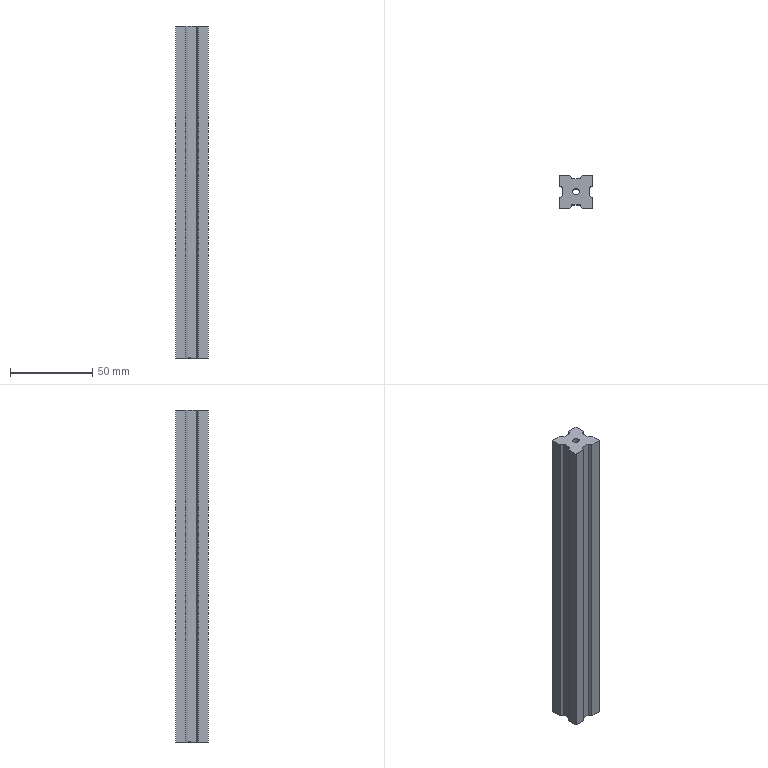Part | SolidWorks | features CirPattern 1, Extrusion 1, ICE 1 | 1 solid | 24 faces | box 20 x 20 x 202 mm | volume 68046 mm3 | plane 22 | cylinder 2 | commonest cylinder face diameters 3.889 x2
STEP:
#1=CARTESIAN_POINT('',(-1.944,0.,101.));
#2=VERTEX_POINT('',#1);
#3=CARTESIAN_POINT('',(1.944,0.,101.));
#4=VERTEX_POINT('',#3);
#5=CARTESIAN_POINT('',(0.,0.,101.));
#6=DIRECTION('',(0.,0.,1.));
#7=DIRECTION('',(1.,0.,0.));
#8=AXIS2_PLACEMENT_3D('',#5,#6,#7);
#9=CIRCLE('',#8,1.944);
#10=EDGE_CURVE('',#2,#4,#9,.T.);
#11=ORIENTED_EDGE('',*,*,#10,.T.);
#12=CARTESIAN_POINT('',(1.944,0.,-101.));
#13=VERTEX_POINT('',#12);
#14=CARTESIAN_POINT('',(1.944,0.,101.));
#15=DIRECTION('',(0.,0.,-1.));
#16=VECTOR('',#15,1000.);
#17=LINE('',#14,#16);
#18=EDGE_CURVE('',#4,#13,#17,.T.);
#19=ORIENTED_EDGE('',*,*,#18,.T.);
#20=CARTESIAN_POINT('',(-1.944,0.,-101.));
#21=VERTEX_POINT('',#20);
#22=CARTESIAN_POINT('',(0.,0.,-101.));
#23=DIRECTION('',(0.,0.,1.));
#24=DIRECTION('',(1.,0.,0.));
#25=AXIS2_PLACEMENT_3D('',#22,#23,#24);
#26=CIRCLE('',#25,1.944);
#27=EDGE_CURVE('',#21,#13,#26,.T.);
#28=ORIENTED_EDGE('',*,*,#27,.F.);
#29=CARTESIAN_POINT('',(-1.944,0.,101.));
#30=DIRECTION('',(0.,0.,-1.));
#31=VECTOR('',#30,1000.);
#32=LINE('',#29,#31);
#33=EDGE_CURVE('',#2,#21,#32,.T.);
#34=ORIENTED_EDGE('',*,*,#33,.F.);
#35=EDGE_LOOP('',(#11,#19,#28,#34));
#36=FACE_OUTER_BOUND('',#35,.T.);
#37=CARTESIAN_POINT('',(0.,0.,101.));
#38=DIRECTION('',(0.,0.,-1.));
#39=DIRECTION('',(-1.,0.,0.));
#40=AXIS2_PLACEMENT_3D('',#37,#38,#39);
#41=CYLINDRICAL_SURFACE('',#40,1.944);
#42=ADVANCED_FACE('',(#36),#41,.F.);
#43=CARTESIAN_POINT('',(-10.,3.694,101.));
#44=VERTEX_POINT('',#43);
#45=CARTESIAN_POINT('',(-10.,3.694,-101.));
#46=VERTEX_POINT('',#45);
#47=CARTESIAN_POINT('',(-10.,3.694,355.963));
#48=DIRECTION('',(0.,0.,-1.));
#49=VECTOR('',#48,1000.);
#50=LINE('',#47,#49);
#51=EDGE_CURVE('',#44,#46,#50,.T.);
#52=ORIENTED_EDGE('',*,*,#51,.F.);
#53=CARTESIAN_POINT('',(-10.,10.,101.));
#54=VERTEX_POINT('',#53);
#55=CARTESIAN_POINT('',(-10.,-10.,101.));
#56=DIRECTION('',(0.,-1.,0.));
#57=VECTOR('',#56,1000.);
#58=LINE('',#55,#57);
#59=EDGE_CURVE('',#54,#44,#58,.T.);
#60=ORIENTED_EDGE('',*,*,#59,.F.);
#61=CARTESIAN_POINT('',(-10.,10.,-101.));
#62=VERTEX_POINT('',#61);
#63=CARTESIAN_POINT('',(-10.,10.,101.));
#64=DIRECTION('',(0.,0.,-1.));
#65=VECTOR('',#64,1000.);
#66=LINE('',#63,#65);
#67=EDGE_CURVE('',#54,#62,#66,.T.);
#68=ORIENTED_EDGE('',*,*,#67,.T.);
#69=CARTESIAN_POINT('',(-10.,-10.,-101.));
#70=DIRECTION('',(0.,-1.,0.));
#71=VECTOR('',#70,1000.);
#72=LINE('',#69,#71);
#73=EDGE_CURVE('',#62,#46,#72,.T.);
#74=ORIENTED_EDGE('',*,*,#73,.T.);
#75=EDGE_LOOP('',(#52,#60,#68,#74));
#76=FACE_OUTER_BOUND('',#75,.T.);
#77=CARTESIAN_POINT('',(-10.,-10.,101.));
#78=DIRECTION('',(1.,0.,0.));
#79=DIRECTION('',(0.,0.,-1.));
#80=AXIS2_PLACEMENT_3D('',#77,#78,#79);
#81=PLANE('',#80);
#82=ADVANCED_FACE('',(#76),#81,.F.);
#83=ORIENTED_EDGE('',*,*,#10,.F.);
#84=CARTESIAN_POINT('',(0.,0.,101.));
#85=DIRECTION('',(0.,0.,1.));
#86=DIRECTION('',(1.,0.,0.));
#87=AXIS2_PLACEMENT_3D('',#84,#85,#86);
#88=CIRCLE('',#87,1.944);
#89=EDGE_CURVE('',#4,#2,#88,.T.);
#90=ORIENTED_EDGE('',*,*,#89,.F.);
#91=EDGE_LOOP('',(#83,#90));
#92=FACE_BOUND('',#91,.T.);
#93=CARTESIAN_POINT('',(-7.931,2.5,101.));
#94=VERTEX_POINT('',#93);
#95=CARTESIAN_POINT('',(-7.931,-2.5,101.));
#96=VERTEX_POINT('',#95);
#97=CARTESIAN_POINT('',(-7.931,0.,101.));
#98=DIRECTION('',(0.,-1.,0.));
#99=VECTOR('',#98,1000.);
#100=LINE('',#97,#99);
#101=EDGE_CURVE('',#94,#96,#100,.T.);
#102=ORIENTED_EDGE('',*,*,#101,.T.);
#103=CARTESIAN_POINT('',(-10.,-3.694,101.));
#104=VERTEX_POINT('',#103);
#105=CARTESIAN_POINT('',(-0.9003,1.559,101.));
#106=DIRECTION('',(-0.866,-0.5,0.));
#107=VECTOR('',#106,1000.);
#108=LINE('',#105,#107);
#109=EDGE_CURVE('',#96,#104,#108,.T.);
#110=ORIENTED_EDGE('',*,*,#109,.T.);
#111=CARTESIAN_POINT('',(-10.,-10.,101.));
#112=VERTEX_POINT('',#111);
#113=CARTESIAN_POINT('',(-10.,-10.,101.));
#114=DIRECTION('',(0.,-1.,0.));
#115=VECTOR('',#114,1000.);
#116=LINE('',#113,#115);
#117=EDGE_CURVE('',#104,#112,#116,.T.);
#118=ORIENTED_EDGE('',*,*,#117,.T.);
#119=CARTESIAN_POINT('',(-3.694,-10.,101.));
#120=VERTEX_POINT('',#119);
#121=CARTESIAN_POINT('',(10.,-10.,101.));
#122=DIRECTION('',(1.,0.,0.));
#123=VECTOR('',#122,1000.);
#124=LINE('',#121,#123);
#125=EDGE_CURVE('',#112,#120,#124,.T.);
#126=ORIENTED_EDGE('',*,*,#125,.T.);
#127=CARTESIAN_POINT('',(-2.5,-7.931,101.));
#128=VERTEX_POINT('',#127);
#129=CARTESIAN_POINT('',(1.559,-0.9003,101.));
#130=DIRECTION('',(0.5,0.866,0.));
#131=VECTOR('',#130,1000.);
#132=LINE('',#129,#131);
#133=EDGE_CURVE('',#120,#128,#132,.T.);
#134=ORIENTED_EDGE('',*,*,#133,.T.);
#135=CARTESIAN_POINT('',(2.5,-7.931,101.));
#136=VERTEX_POINT('',#135);
#137=CARTESIAN_POINT('',(0.,-7.931,101.));
#138=DIRECTION('',(1.,0.,0.));
#139=VECTOR('',#138,1000.);
#140=LINE('',#137,#139);
#141=EDGE_CURVE('',#128,#136,#140,.T.);
#142=ORIENTED_EDGE('',*,*,#141,.T.);
#143=CARTESIAN_POINT('',(3.694,-10.,101.));
#144=VERTEX_POINT('',#143);
#145=CARTESIAN_POINT('',(-1.559,-0.9003,101.));
#146=DIRECTION('',(0.5,-0.866,0.));
#147=VECTOR('',#146,1000.);
#148=LINE('',#145,#147);
#149=EDGE_CURVE('',#136,#144,#148,.T.);
#150=ORIENTED_EDGE('',*,*,#149,.T.);
#151=CARTESIAN_POINT('',(10.,-10.,101.));
#152=VERTEX_POINT('',#151);
#153=CARTESIAN_POINT('',(10.,-10.,101.));
#154=DIRECTION('',(1.,0.,0.));
#155=VECTOR('',#154,1000.);
#156=LINE('',#153,#155);
#157=EDGE_CURVE('',#144,#152,#156,.T.);
#158=ORIENTED_EDGE('',*,*,#157,.T.);
#159=CARTESIAN_POINT('',(10.,-3.694,101.));
#160=VERTEX_POINT('',#159);
#161=CARTESIAN_POINT('',(10.,-10.,101.));
#162=DIRECTION('',(0.,1.,0.));
#163=VECTOR('',#162,1000.);
#164=LINE('',#161,#163);
#165=EDGE_CURVE('',#152,#160,#164,.T.);
#166=ORIENTED_EDGE('',*,*,#165,.T.);
#167=CARTESIAN_POINT('',(7.931,-2.5,101.));
#168=VERTEX_POINT('',#167);
#169=CARTESIAN_POINT('',(0.9003,1.559,101.));
#170=DIRECTION('',(-0.866,0.5,0.));
#171=VECTOR('',#170,1000.);
#172=LINE('',#169,#171);
#173=EDGE_CURVE('',#160,#168,#172,.T.);
#174=ORIENTED_EDGE('',*,*,#173,.T.);
#175=CARTESIAN_POINT('',(7.931,2.5,101.));
#176=VERTEX_POINT('',#175);
#177=CARTESIAN_POINT('',(7.931,0.,101.));
#178=DIRECTION('',(0.,1.,0.));
#179=VECTOR('',#178,1000.);
#180=LINE('',#177,#179);
#181=EDGE_CURVE('',#168,#176,#180,.T.);
#182=ORIENTED_EDGE('',*,*,#181,.T.);
#183=CARTESIAN_POINT('',(10.,3.694,101.));
#184=VERTEX_POINT('',#183);
#185=CARTESIAN_POINT('',(0.9003,-1.559,101.));
#186=DIRECTION('',(0.866,0.5,0.));
#187=VECTOR('',#186,1000.);
#188=LINE('',#185,#187);
#189=EDGE_CURVE('',#176,#184,#188,.T.);
#190=ORIENTED_EDGE('',*,*,#189,.T.);
#191=CARTESIAN_POINT('',(10.,10.,101.));
#192=VERTEX_POINT('',#191);
#193=CARTESIAN_POINT('',(10.,-10.,101.));
#194=DIRECTION('',(0.,1.,0.));
#195=VECTOR('',#194,1000.);
#196=LINE('',#193,#195);
#197=EDGE_CURVE('',#184,#192,#196,.T.);
#198=ORIENTED_EDGE('',*,*,#197,.T.);
#199=CARTESIAN_POINT('',(3.694,10.,101.));
#200=VERTEX_POINT('',#199);
#201=CARTESIAN_POINT('',(10.,10.,101.));
#202=DIRECTION('',(-1.,0.,0.));
#203=VECTOR('',#202,1000.);
#204=LINE('',#201,#203);
#205=EDGE_CURVE('',#192,#200,#204,.T.);
#206=ORIENTED_EDGE('',*,*,#205,.T.);
#207=CARTESIAN_POINT('',(2.5,7.931,101.));
#208=VERTEX_POINT('',#207);
#209=CARTESIAN_POINT('',(-1.559,0.9003,101.));
#210=DIRECTION('',(-0.5,-0.866,0.));
#211=VECTOR('',#210,1000.);
#212=LINE('',#209,#211);
#213=EDGE_CURVE('',#200,#208,#212,.T.);
#214=ORIENTED_EDGE('',*,*,#213,.T.);
#215=CARTESIAN_POINT('',(-2.5,7.931,101.));
#216=VERTEX_POINT('',#215);
#217=CARTESIAN_POINT('',(0.,7.931,101.));
#218=DIRECTION('',(-1.,0.,0.));
#219=VECTOR('',#218,1000.);
#220=LINE('',#217,#219);
#221=EDGE_CURVE('',#208,#216,#220,.T.);
#222=ORIENTED_EDGE('',*,*,#221,.T.);
#223=CARTESIAN_POINT('',(-3.694,10.,101.));
#224=VERTEX_POINT('',#223);
#225=CARTESIAN_POINT('',(1.559,0.9003,101.));
#226=DIRECTION('',(-0.5,0.866,0.));
#227=VECTOR('',#226,1000.);
#228=LINE('',#225,#227);
#229=EDGE_CURVE('',#216,#224,#228,.T.);
#230=ORIENTED_EDGE('',*,*,#229,.T.);
#231=CARTESIAN_POINT('',(10.,10.,101.));
#232=DIRECTION('',(-1.,0.,0.));
#233=VECTOR('',#232,1000.);
#234=LINE('',#231,#233);
#235=EDGE_CURVE('',#224,#54,#234,.T.);
#236=ORIENTED_EDGE('',*,*,#235,.T.);
#237=ORIENTED_EDGE('',*,*,#59,.T.);
#238=CARTESIAN_POINT('',(-0.9003,-1.559,101.));
#239=DIRECTION('',(0.866,-0.5,0.));
#240=VECTOR('',#239,1000.);
#241=LINE('',#238,#240);
#242=EDGE_CURVE('',#44,#94,#241,.T.);
#243=ORIENTED_EDGE('',*,*,#242,.T.);
#244=EDGE_LOOP('',(#102,#110,#118,#126,#134,#142,#150,#158,#166,#174,#182,#190,#198,#206,#214,#222,#230,#236,#237,#243));
#245=FACE_OUTER_BOUND('',#244,.T.);
#246=CARTESIAN_POINT('',(0.,0.,101.));
#247=DIRECTION('',(0.,0.,1.));
#248=DIRECTION('',(1.,0.,0.));
#249=AXIS2_PLACEMENT_3D('',#246,#247,#248);
#250=PLANE('',#249);
#251=ADVANCED_FACE('',(#92,#245),#250,.T.);
#252=ORIENTED_EDGE('',*,*,#27,.T.);
#253=CARTESIAN_POINT('',(0.,0.,-101.));
#254=DIRECTION('',(0.,0.,1.));
#255=DIRECTION('',(1.,0.,0.));
#256=AXIS2_PLACEMENT_3D('',#253,#254,#255);
#257=CIRCLE('',#256,1.944);
#258=EDGE_CURVE('',#13,#21,#257,.T.);
#259=ORIENTED_EDGE('',*,*,#258,.T.);
#260=EDGE_LOOP('',(#252,#259));
#261=FACE_BOUND('',#260,.T.);
#262=CARTESIAN_POINT('',(-7.931,-2.5,-101.));
#263=VERTEX_POINT('',#262);
#264=CARTESIAN_POINT('',(-10.,-3.694,-101.));
#265=VERTEX_POINT('',#264);
#266=CARTESIAN_POINT('',(-0.9003,1.559,-101.));
#267=DIRECTION('',(-0.866,-0.5,0.));
#268=VECTOR('',#267,1000.);
#269=LINE('',#266,#268);
#270=EDGE_CURVE('',#263,#265,#269,.T.);
#271=ORIENTED_EDGE('',*,*,#270,.F.);
#272=CARTESIAN_POINT('',(-7.931,2.5,-101.));
#273=VERTEX_POINT('',#272);
#274=CARTESIAN_POINT('',(-7.931,0.,-101.));
#275=DIRECTION('',(0.,-1.,0.));
#276=VECTOR('',#275,1000.);
#277=LINE('',#274,#276);
#278=EDGE_CURVE('',#273,#263,#277,.T.);
#279=ORIENTED_EDGE('',*,*,#278,.F.);
#280=CARTESIAN_POINT('',(-0.9003,-1.559,-101.));
#281=DIRECTION('',(0.866,-0.5,0.));
#282=VECTOR('',#281,1000.);
#283=LINE('',#280,#282);
#284=EDGE_CURVE('',#46,#273,#283,.T.);
#285=ORIENTED_EDGE('',*,*,#284,.F.);
#286=ORIENTED_EDGE('',*,*,#73,.F.);
#287=CARTESIAN_POINT('',(-3.694,10.,-101.));
#288=VERTEX_POINT('',#287);
#289=CARTESIAN_POINT('',(10.,10.,-101.));
#290=DIRECTION('',(-1.,0.,0.));
#291=VECTOR('',#290,1000.);
#292=LINE('',#289,#291);
#293=EDGE_CURVE('',#288,#62,#292,.T.);
#294=ORIENTED_EDGE('',*,*,#293,.F.);
#295=CARTESIAN_POINT('',(-2.5,7.931,-101.));
#296=VERTEX_POINT('',#295);
#297=CARTESIAN_POINT('',(1.559,0.9003,-101.));
#298=DIRECTION('',(-0.5,0.866,0.));
#299=VECTOR('',#298,1000.);
#300=LINE('',#297,#299);
#301=EDGE_CURVE('',#296,#288,#300,.T.);
#302=ORIENTED_EDGE('',*,*,#301,.F.);
#303=CARTESIAN_POINT('',(2.5,7.931,-101.));
#304=VERTEX_POINT('',#303);
#305=CARTESIAN_POINT('',(0.,7.931,-101.));
#306=DIRECTION('',(-1.,0.,0.));
#307=VECTOR('',#306,1000.);
#308=LINE('',#305,#307);
#309=EDGE_CURVE('',#304,#296,#308,.T.);
#310=ORIENTED_EDGE('',*,*,#309,.F.);
#311=CARTESIAN_POINT('',(3.694,10.,-101.));
#312=VERTEX_POINT('',#311);
#313=CARTESIAN_POINT('',(-1.559,0.9003,-101.));
#314=DIRECTION('',(-0.5,-0.866,0.));
#315=VECTOR('',#314,1000.);
#316=LINE('',#313,#315);
#317=EDGE_CURVE('',#312,#304,#316,.T.);
#318=ORIENTED_EDGE('',*,*,#317,.F.);
#319=CARTESIAN_POINT('',(10.,10.,-101.));
#320=VERTEX_POINT('',#319);
#321=CARTESIAN_POINT('',(10.,10.,-101.));
#322=DIRECTION('',(-1.,0.,0.));
#323=VECTOR('',#322,1000.);
#324=LINE('',#321,#323);
#325=EDGE_CURVE('',#320,#312,#324,.T.);
#326=ORIENTED_EDGE('',*,*,#325,.F.);
#327=CARTESIAN_POINT('',(10.,3.694,-101.));
#328=VERTEX_POINT('',#327);
#329=CARTESIAN_POINT('',(10.,-10.,-101.));
#330=DIRECTION('',(0.,1.,0.));
#331=VECTOR('',#330,1000.);
#332=LINE('',#329,#331);
#333=EDGE_CURVE('',#328,#320,#332,.T.);
#334=ORIENTED_EDGE('',*,*,#333,.F.);
#335=CARTESIAN_POINT('',(7.931,2.5,-101.));
#336=VERTEX_POINT('',#335);
#337=CARTESIAN_POINT('',(0.9003,-1.559,-101.));
#338=DIRECTION('',(0.866,0.5,0.));
#339=VECTOR('',#338,1000.);
#340=LINE('',#337,#339);
#341=EDGE_CURVE('',#336,#328,#340,.T.);
#342=ORIENTED_EDGE('',*,*,#341,.F.);
#343=CARTESIAN_POINT('',(7.931,-2.5,-101.));
#344=VERTEX_POINT('',#343);
#345=CARTESIAN_POINT('',(7.931,0.,-101.));
#346=DIRECTION('',(0.,1.,0.));
#347=VECTOR('',#346,1000.);
#348=LINE('',#345,#347);
#349=EDGE_CURVE('',#344,#336,#348,.T.);
#350=ORIENTED_EDGE('',*,*,#349,.F.);
#351=CARTESIAN_POINT('',(10.,-3.694,-101.));
#352=VERTEX_POINT('',#351);
#353=CARTESIAN_POINT('',(0.9003,1.559,-101.));
#354=DIRECTION('',(-0.866,0.5,0.));
#355=VECTOR('',#354,1000.);
#356=LINE('',#353,#355);
#357=EDGE_CURVE('',#352,#344,#356,.T.);
#358=ORIENTED_EDGE('',*,*,#357,.F.);
#359=CARTESIAN_POINT('',(10.,-10.,-101.));
#360=VERTEX_POINT('',#359);
#361=CARTESIAN_POINT('',(10.,-10.,-101.));
#362=DIRECTION('',(0.,1.,0.));
#363=VECTOR('',#362,1000.);
#364=LINE('',#361,#363);
#365=EDGE_CURVE('',#360,#352,#364,.T.);
#366=ORIENTED_EDGE('',*,*,#365,.F.);
#367=CARTESIAN_POINT('',(3.694,-10.,-101.));
#368=VERTEX_POINT('',#367);
#369=CARTESIAN_POINT('',(10.,-10.,-101.));
#370=DIRECTION('',(1.,0.,0.));
#371=VECTOR('',#370,1000.);
#372=LINE('',#369,#371);
#373=EDGE_CURVE('',#368,#360,#372,.T.);
#374=ORIENTED_EDGE('',*,*,#373,.F.);
#375=CARTESIAN_POINT('',(2.5,-7.931,-101.));
#376=VERTEX_POINT('',#375);
#377=CARTESIAN_POINT('',(-1.559,-0.9003,-101.));
#378=DIRECTION('',(0.5,-0.866,0.));
#379=VECTOR('',#378,1000.);
#380=LINE('',#377,#379);
#381=EDGE_CURVE('',#376,#368,#380,.T.);
#382=ORIENTED_EDGE('',*,*,#381,.F.);
#383=CARTESIAN_POINT('',(-2.5,-7.931,-101.));
#384=VERTEX_POINT('',#383);
#385=CARTESIAN_POINT('',(0.,-7.931,-101.));
#386=DIRECTION('',(1.,0.,0.));
#387=VECTOR('',#386,1000.);
#388=LINE('',#385,#387);
#389=EDGE_CURVE('',#384,#376,#388,.T.);
#390=ORIENTED_EDGE('',*,*,#389,.F.);
#391=CARTESIAN_POINT('',(-3.694,-10.,-101.));
#392=VERTEX_POINT('',#391);
#393=CARTESIAN_POINT('',(1.559,-0.9003,-101.));
#394=DIRECTION('',(0.5,0.866,0.));
#395=VECTOR('',#394,1000.);
#396=LINE('',#393,#395);
#397=EDGE_CURVE('',#392,#384,#396,.T.);
#398=ORIENTED_EDGE('',*,*,#397,.F.);
#399=CARTESIAN_POINT('',(-10.,-10.,-101.));
#400=VERTEX_POINT('',#399);
#401=CARTESIAN_POINT('',(10.,-10.,-101.));
#402=DIRECTION('',(1.,0.,0.));
#403=VECTOR('',#402,1000.);
#404=LINE('',#401,#403);
#405=EDGE_CURVE('',#400,#392,#404,.T.);
#406=ORIENTED_EDGE('',*,*,#405,.F.);
#407=CARTESIAN_POINT('',(-10.,-10.,-101.));
#408=DIRECTION('',(0.,-1.,0.));
#409=VECTOR('',#408,1000.);
#410=LINE('',#407,#409);
#411=EDGE_CURVE('',#265,#400,#410,.T.);
#412=ORIENTED_EDGE('',*,*,#411,.F.);
#413=EDGE_LOOP('',(#271,#279,#285,#286,#294,#302,#310,#318,#326,#334,#342,#350,#358,#366,#374,#382,#390,#398,#406,#412));
#414=FACE_OUTER_BOUND('',#413,.T.);
#415=CARTESIAN_POINT('',(0.,0.,-101.));
#416=DIRECTION('',(0.,0.,1.));
#417=DIRECTION('',(1.,0.,0.));
#418=AXIS2_PLACEMENT_3D('',#415,#416,#417);
#419=PLANE('',#418);
#420=ADVANCED_FACE('',(#261,#414),#419,.F.);
#421=CARTESIAN_POINT('',(-3.694,-10.,355.963));
#422=DIRECTION('',(0.,0.,-1.));
#423=VECTOR('',#422,1000.);
#424=LINE('',#421,#423);
#425=EDGE_CURVE('',#120,#392,#424,.T.);
#426=ORIENTED_EDGE('',*,*,#425,.F.);
#427=ORIENTED_EDGE('',*,*,#125,.F.);
#428=CARTESIAN_POINT('',(-10.,-10.,101.));
#429=DIRECTION('',(0.,0.,-1.));
#430=VECTOR('',#429,1000.);
#431=LINE('',#428,#430);
#432=EDGE_CURVE('',#112,#400,#431,.T.);
#433=ORIENTED_EDGE('',*,*,#432,.T.);
#434=ORIENTED_EDGE('',*,*,#405,.T.);
#435=EDGE_LOOP('',(#426,#427,#433,#434));
#436=FACE_OUTER_BOUND('',#435,.T.);
#437=CARTESIAN_POINT('',(10.,-10.,101.));
#438=DIRECTION('',(0.,1.,0.));
#439=DIRECTION('',(-1.,0.,0.));
#440=AXIS2_PLACEMENT_3D('',#437,#438,#439);
#441=PLANE('',#440);
#442=ADVANCED_FACE('',(#436),#441,.F.);
#443=CARTESIAN_POINT('',(10.,-3.694,355.963));
#444=DIRECTION('',(0.,0.,-1.));
#445=VECTOR('',#444,1000.);
#446=LINE('',#443,#445);
#447=EDGE_CURVE('',#160,#352,#446,.T.);
#448=ORIENTED_EDGE('',*,*,#447,.F.);
#449=ORIENTED_EDGE('',*,*,#165,.F.);
#450=CARTESIAN_POINT('',(10.,-10.,101.));
#451=DIRECTION('',(0.,0.,-1.));
#452=VECTOR('',#451,1000.);
#453=LINE('',#450,#452);
#454=EDGE_CURVE('',#152,#360,#453,.T.);
#455=ORIENTED_EDGE('',*,*,#454,.T.);
#456=ORIENTED_EDGE('',*,*,#365,.T.);
#457=EDGE_LOOP('',(#448,#449,#455,#456));
#458=FACE_OUTER_BOUND('',#457,.T.);
#459=CARTESIAN_POINT('',(10.,-10.,101.));
#460=DIRECTION('',(-1.,0.,0.));
#461=DIRECTION('',(0.,0.,1.));
#462=AXIS2_PLACEMENT_3D('',#459,#460,#461);
#463=PLANE('',#462);
#464=ADVANCED_FACE('',(#458),#463,.F.);
#465=CARTESIAN_POINT('',(3.694,10.,355.963));
#466=DIRECTION('',(0.,0.,-1.));
#467=VECTOR('',#466,1000.);
#468=LINE('',#465,#467);
#469=EDGE_CURVE('',#200,#312,#468,.T.);
#470=ORIENTED_EDGE('',*,*,#469,.F.);
#471=ORIENTED_EDGE('',*,*,#205,.F.);
#472=CARTESIAN_POINT('',(10.,10.,101.));
#473=DIRECTION('',(0.,0.,-1.));
#474=VECTOR('',#473,1000.);
#475=LINE('',#472,#474);
#476=EDGE_CURVE('',#192,#320,#475,.T.);
#477=ORIENTED_EDGE('',*,*,#476,.T.);
#478=ORIENTED_EDGE('',*,*,#325,.T.);
#479=EDGE_LOOP('',(#470,#471,#477,#478));
#480=FACE_OUTER_BOUND('',#479,.T.);
#481=CARTESIAN_POINT('',(10.,10.,101.));
#482=DIRECTION('',(0.,-1.,0.));
#483=DIRECTION('',(1.,0.,0.));
#484=AXIS2_PLACEMENT_3D('',#481,#482,#483);
#485=PLANE('',#484);
#486=ADVANCED_FACE('',(#480),#485,.F.);
#487=ORIENTED_EDGE('',*,*,#117,.F.);
#488=CARTESIAN_POINT('',(-10.,-3.694,355.963));
#489=DIRECTION('',(0.,0.,-1.));
#490=VECTOR('',#489,1000.);
#491=LINE('',#488,#490);
#492=EDGE_CURVE('',#104,#265,#491,.T.);
#493=ORIENTED_EDGE('',*,*,#492,.T.);
#494=ORIENTED_EDGE('',*,*,#411,.T.);
#495=ORIENTED_EDGE('',*,*,#432,.F.);
#496=EDGE_LOOP('',(#487,#493,#494,#495));
#497=FACE_OUTER_BOUND('',#496,.T.);
#498=CARTESIAN_POINT('',(-10.,-10.,101.));
#499=DIRECTION('',(1.,0.,0.));
#500=DIRECTION('',(0.,0.,-1.));
#501=AXIS2_PLACEMENT_3D('',#498,#499,#500);
#502=PLANE('',#501);
#503=ADVANCED_FACE('',(#497),#502,.F.);
#504=ORIENTED_EDGE('',*,*,#157,.F.);
#505=CARTESIAN_POINT('',(3.694,-10.,355.963));
#506=DIRECTION('',(0.,0.,-1.));
#507=VECTOR('',#506,1000.);
#508=LINE('',#505,#507);
#509=EDGE_CURVE('',#144,#368,#508,.T.);
#510=ORIENTED_EDGE('',*,*,#509,.T.);
#511=ORIENTED_EDGE('',*,*,#373,.T.);
#512=ORIENTED_EDGE('',*,*,#454,.F.);
#513=EDGE_LOOP('',(#504,#510,#511,#512));
#514=FACE_OUTER_BOUND('',#513,.T.);
#515=CARTESIAN_POINT('',(10.,-10.,101.));
#516=DIRECTION('',(0.,1.,0.));
#517=DIRECTION('',(-1.,0.,0.));
#518=AXIS2_PLACEMENT_3D('',#515,#516,#517);
#519=PLANE('',#518);
#520=ADVANCED_FACE('',(#514),#519,.F.);
#521=ORIENTED_EDGE('',*,*,#197,.F.);
#522=CARTESIAN_POINT('',(10.,3.694,355.963));
#523=DIRECTION('',(0.,0.,-1.));
#524=VECTOR('',#523,1000.);
#525=LINE('',#522,#524);
#526=EDGE_CURVE('',#184,#328,#525,.T.);
#527=ORIENTED_EDGE('',*,*,#526,.T.);
#528=ORIENTED_EDGE('',*,*,#333,.T.);
#529=ORIENTED_EDGE('',*,*,#476,.F.);
#530=EDGE_LOOP('',(#521,#527,#528,#529));
#531=FACE_OUTER_BOUND('',#530,.T.);
#532=CARTESIAN_POINT('',(10.,-10.,101.));
#533=DIRECTION('',(-1.,0.,0.));
#534=DIRECTION('',(0.,0.,1.));
#535=AXIS2_PLACEMENT_3D('',#532,#533,#534);
#536=PLANE('',#535);
#537=ADVANCED_FACE('',(#531),#536,.F.);
#538=ORIENTED_EDGE('',*,*,#235,.F.);
#539=CARTESIAN_POINT('',(-3.694,10.,355.963));
#540=DIRECTION('',(0.,0.,-1.));
#541=VECTOR('',#540,1000.);
#542=LINE('',#539,#541);
#543=EDGE_CURVE('',#224,#288,#542,.T.);
#544=ORIENTED_EDGE('',*,*,#543,.T.);
#545=ORIENTED_EDGE('',*,*,#293,.T.);
#546=ORIENTED_EDGE('',*,*,#67,.F.);
#547=EDGE_LOOP('',(#538,#544,#545,#546));
#548=FACE_OUTER_BOUND('',#547,.T.);
#549=CARTESIAN_POINT('',(10.,10.,101.));
#550=DIRECTION('',(0.,-1.,0.));
#551=DIRECTION('',(1.,0.,0.));
#552=AXIS2_PLACEMENT_3D('',#549,#550,#551);
#553=PLANE('',#552);
#554=ADVANCED_FACE('',(#548),#553,.F.);
#555=ORIENTED_EDGE('',*,*,#18,.F.);
#556=ORIENTED_EDGE('',*,*,#89,.T.);
#557=ORIENTED_EDGE('',*,*,#33,.T.);
#558=ORIENTED_EDGE('',*,*,#258,.F.);
#559=EDGE_LOOP('',(#555,#556,#557,#558));
#560=FACE_OUTER_BOUND('',#559,.T.);
#561=CARTESIAN_POINT('',(0.,0.,101.));
#562=DIRECTION('',(0.,0.,-1.));
#563=DIRECTION('',(-1.,0.,0.));
#564=AXIS2_PLACEMENT_3D('',#561,#562,#563);
#565=CYLINDRICAL_SURFACE('',#564,1.944);
#566=ADVANCED_FACE('',(#560),#565,.F.);
#567=ORIENTED_EDGE('',*,*,#229,.F.);
#568=CARTESIAN_POINT('',(-2.5,7.931,355.963));
#569=DIRECTION('',(0.,0.,-1.));
#570=VECTOR('',#569,1000.);
#571=LINE('',#568,#570);
#572=EDGE_CURVE('',#216,#296,#571,.T.);
#573=ORIENTED_EDGE('',*,*,#572,.T.);
#574=ORIENTED_EDGE('',*,*,#301,.T.);
#575=ORIENTED_EDGE('',*,*,#543,.F.);
#576=EDGE_LOOP('',(#567,#573,#574,#575));
#577=FACE_OUTER_BOUND('',#576,.T.);
#578=CARTESIAN_POINT('',(-3.694,10.,355.963));
#579=DIRECTION('',(0.866,0.5,0.));
#580=DIRECTION('',(-0.5,0.866,0.));
#581=AXIS2_PLACEMENT_3D('',#578,#579,#580);
#582=PLANE('',#581);
#583=ADVANCED_FACE('',(#577),#582,.T.);
#584=ORIENTED_EDGE('',*,*,#221,.F.);
#585=CARTESIAN_POINT('',(2.5,7.931,355.963));
#586=DIRECTION('',(0.,0.,-1.));
#587=VECTOR('',#586,1000.);
#588=LINE('',#585,#587);
#589=EDGE_CURVE('',#208,#304,#588,.T.);
#590=ORIENTED_EDGE('',*,*,#589,.T.);
#591=ORIENTED_EDGE('',*,*,#309,.T.);
#592=ORIENTED_EDGE('',*,*,#572,.F.);
#593=EDGE_LOOP('',(#584,#590,#591,#592));
#594=FACE_OUTER_BOUND('',#593,.T.);
#595=CARTESIAN_POINT('',(-2.5,7.931,355.963));
#596=DIRECTION('',(0.,1.,0.));
#597=DIRECTION('',(0.,0.,1.));
#598=AXIS2_PLACEMENT_3D('',#595,#596,#597);
#599=PLANE('',#598);
#600=ADVANCED_FACE('',(#594),#599,.T.);
#601=ORIENTED_EDGE('',*,*,#213,.F.);
#602=ORIENTED_EDGE('',*,*,#469,.T.);
#603=ORIENTED_EDGE('',*,*,#317,.T.);
#604=ORIENTED_EDGE('',*,*,#589,.F.);
#605=EDGE_LOOP('',(#601,#602,#603,#604));
#606=FACE_OUTER_BOUND('',#605,.T.);
#607=CARTESIAN_POINT('',(2.5,7.931,355.963));
#608=DIRECTION('',(-0.866,0.5,0.));
#609=DIRECTION('',(-0.5,-0.866,0.));
#610=AXIS2_PLACEMENT_3D('',#607,#608,#609);
#611=PLANE('',#610);
#612=ADVANCED_FACE('',(#606),#611,.T.);
#613=ORIENTED_EDGE('',*,*,#189,.F.);
#614=CARTESIAN_POINT('',(7.931,2.5,355.963));
#615=DIRECTION('',(0.,0.,-1.));
#616=VECTOR('',#615,1000.);
#617=LINE('',#614,#616);
#618=EDGE_CURVE('',#176,#336,#617,.T.);
#619=ORIENTED_EDGE('',*,*,#618,.T.);
#620=ORIENTED_EDGE('',*,*,#341,.T.);
#621=ORIENTED_EDGE('',*,*,#526,.F.);
#622=EDGE_LOOP('',(#613,#619,#620,#621));
#623=FACE_OUTER_BOUND('',#622,.T.);
#624=CARTESIAN_POINT('',(10.,3.694,355.963));
#625=DIRECTION('',(0.5,-0.866,0.));
#626=DIRECTION('',(0.866,0.5,0.));
#627=AXIS2_PLACEMENT_3D('',#624,#625,#626);
#628=PLANE('',#627);
#629=ADVANCED_FACE('',(#623),#628,.T.);
#630=ORIENTED_EDGE('',*,*,#181,.F.);
#631=CARTESIAN_POINT('',(7.931,-2.5,355.963));
#632=DIRECTION('',(0.,0.,-1.));
#633=VECTOR('',#632,1000.);
#634=LINE('',#631,#633);
#635=EDGE_CURVE('',#168,#344,#634,.T.);
#636=ORIENTED_EDGE('',*,*,#635,.T.);
#637=ORIENTED_EDGE('',*,*,#349,.T.);
#638=ORIENTED_EDGE('',*,*,#618,.F.);
#639=EDGE_LOOP('',(#630,#636,#637,#638));
#640=FACE_OUTER_BOUND('',#639,.T.);
#641=CARTESIAN_POINT('',(7.931,2.5,355.963));
#642=DIRECTION('',(1.,0.,0.));
#643=DIRECTION('',(0.,1.,0.));
#644=AXIS2_PLACEMENT_3D('',#641,#642,#643);
#645=PLANE('',#644);
#646=ADVANCED_FACE('',(#640),#645,.T.);
#647=ORIENTED_EDGE('',*,*,#173,.F.);
#648=ORIENTED_EDGE('',*,*,#447,.T.);
#649=ORIENTED_EDGE('',*,*,#357,.T.);
#650=ORIENTED_EDGE('',*,*,#635,.F.);
#651=EDGE_LOOP('',(#647,#648,#649,#650));
#652=FACE_OUTER_BOUND('',#651,.T.);
#653=CARTESIAN_POINT('',(7.931,-2.5,355.963));
#654=DIRECTION('',(0.5,0.866,0.));
#655=DIRECTION('',(-0.866,0.5,0.));
#656=AXIS2_PLACEMENT_3D('',#653,#654,#655);
#657=PLANE('',#656);
#658=ADVANCED_FACE('',(#652),#657,.T.);
#659=ORIENTED_EDGE('',*,*,#149,.F.);
#660=CARTESIAN_POINT('',(2.5,-7.931,355.963));
#661=DIRECTION('',(0.,0.,-1.));
#662=VECTOR('',#661,1000.);
#663=LINE('',#660,#662);
#664=EDGE_CURVE('',#136,#376,#663,.T.);
#665=ORIENTED_EDGE('',*,*,#664,.T.);
#666=ORIENTED_EDGE('',*,*,#381,.T.);
#667=ORIENTED_EDGE('',*,*,#509,.F.);
#668=EDGE_LOOP('',(#659,#665,#666,#667));
#669=FACE_OUTER_BOUND('',#668,.T.);
#670=CARTESIAN_POINT('',(3.694,-10.,355.963));
#671=DIRECTION('',(-0.866,-0.5,0.));
#672=DIRECTION('',(0.5,-0.866,0.));
#673=AXIS2_PLACEMENT_3D('',#670,#671,#672);
#674=PLANE('',#673);
#675=ADVANCED_FACE('',(#669),#674,.T.);
#676=ORIENTED_EDGE('',*,*,#141,.F.);
#677=CARTESIAN_POINT('',(-2.5,-7.931,355.963));
#678=DIRECTION('',(0.,0.,-1.));
#679=VECTOR('',#678,1000.);
#680=LINE('',#677,#679);
#681=EDGE_CURVE('',#128,#384,#680,.T.);
#682=ORIENTED_EDGE('',*,*,#681,.T.);
#683=ORIENTED_EDGE('',*,*,#389,.T.);
#684=ORIENTED_EDGE('',*,*,#664,.F.);
#685=EDGE_LOOP('',(#676,#682,#683,#684));
#686=FACE_OUTER_BOUND('',#685,.T.);
#687=CARTESIAN_POINT('',(2.5,-7.931,355.963));
#688=DIRECTION('',(0.,-1.,0.));
#689=DIRECTION('',(0.,0.,-1.));
#690=AXIS2_PLACEMENT_3D('',#687,#688,#689);
#691=PLANE('',#690);
#692=ADVANCED_FACE('',(#686),#691,.T.);
#693=ORIENTED_EDGE('',*,*,#133,.F.);
#694=ORIENTED_EDGE('',*,*,#425,.T.);
#695=ORIENTED_EDGE('',*,*,#397,.T.);
#696=ORIENTED_EDGE('',*,*,#681,.F.);
#697=EDGE_LOOP('',(#693,#694,#695,#696));
#698=FACE_OUTER_BOUND('',#697,.T.);
#699=CARTESIAN_POINT('',(-2.5,-7.931,355.963));
#700=DIRECTION('',(0.866,-0.5,0.));
#701=DIRECTION('',(0.5,0.866,0.));
#702=AXIS2_PLACEMENT_3D('',#699,#700,#701);
#703=PLANE('',#702);
#704=ADVANCED_FACE('',(#698),#703,.T.);
#705=ORIENTED_EDGE('',*,*,#109,.F.);
#706=CARTESIAN_POINT('',(-7.931,-2.5,355.963));
#707=DIRECTION('',(0.,0.,-1.));
#708=VECTOR('',#707,1000.);
#709=LINE('',#706,#708);
#710=EDGE_CURVE('',#96,#263,#709,.T.);
#711=ORIENTED_EDGE('',*,*,#710,.T.);
#712=ORIENTED_EDGE('',*,*,#270,.T.);
#713=ORIENTED_EDGE('',*,*,#492,.F.);
#714=EDGE_LOOP('',(#705,#711,#712,#713));
#715=FACE_OUTER_BOUND('',#714,.T.);
#716=CARTESIAN_POINT('',(-10.,-3.694,355.963));
#717=DIRECTION('',(-0.5,0.866,0.));
#718=DIRECTION('',(-0.866,-0.5,0.));
#719=AXIS2_PLACEMENT_3D('',#716,#717,#718);
#720=PLANE('',#719);
#721=ADVANCED_FACE('',(#715),#720,.T.);
#722=ORIENTED_EDGE('',*,*,#101,.F.);
#723=CARTESIAN_POINT('',(-7.931,2.5,355.963));
#724=DIRECTION('',(0.,0.,-1.));
#725=VECTOR('',#724,1000.);
#726=LINE('',#723,#725);
#727=EDGE_CURVE('',#94,#273,#726,.T.);
#728=ORIENTED_EDGE('',*,*,#727,.T.);
#729=ORIENTED_EDGE('',*,*,#278,.T.);
#730=ORIENTED_EDGE('',*,*,#710,.F.);
#731=EDGE_LOOP('',(#722,#728,#729,#730));
#732=FACE_OUTER_BOUND('',#731,.T.);
#733=CARTESIAN_POINT('',(-7.931,-2.5,355.963));
#734=DIRECTION('',(-1.,0.,0.));
#735=DIRECTION('',(0.,-1.,0.));
#736=AXIS2_PLACEMENT_3D('',#733,#734,#735);
#737=PLANE('',#736);
#738=ADVANCED_FACE('',(#732),#737,.T.);
#739=ORIENTED_EDGE('',*,*,#242,.F.);
#740=ORIENTED_EDGE('',*,*,#51,.T.);
#741=ORIENTED_EDGE('',*,*,#284,.T.);
#742=ORIENTED_EDGE('',*,*,#727,.F.);
#743=EDGE_LOOP('',(#739,#740,#741,#742));
#744=FACE_OUTER_BOUND('',#743,.T.);
#745=CARTESIAN_POINT('',(-7.931,2.5,355.963));
#746=DIRECTION('',(-0.5,-0.866,0.));
#747=DIRECTION('',(0.866,-0.5,0.));
#748=AXIS2_PLACEMENT_3D('',#745,#746,#747);
#749=PLANE('',#748);
#750=ADVANCED_FACE('',(#744),#749,.T.);
#751=CLOSED_SHELL('',(#42,#82,#251,#420,#442,#464,#486,#503,#520,#537,#554,#566,#583,#600,#612,#629,#646,#658,#675,#692,#704,#721,#738,#750));
#752=MANIFOLD_SOLID_BREP('',#751);
#753=CARTESIAN_POINT('',(0.,0.,0.));
#754=DIRECTION('',(0.,0.,1.));
#755=DIRECTION('',(1.,0.,0.));
#756=AXIS2_PLACEMENT_3D('',#753,#754,#755);
#757=(LENGTH_UNIT()NAMED_UNIT(*)SI_UNIT(.MILLI.,.METRE.));
#758=UNCERTAINTY_MEASURE_WITH_UNIT(LENGTH_MEASURE(0.00001),#757,'','');
#759=(NAMED_UNIT(*)PLANE_ANGLE_UNIT()SI_UNIT($,.RADIAN.));
#760=(NAMED_UNIT(*)SI_UNIT($,.STERADIAN.)SOLID_ANGLE_UNIT());
#761=(GEOMETRIC_REPRESENTATION_CONTEXT(3)GLOBAL_UNCERTAINTY_ASSIGNED_CONTEXT((#758))GLOBAL_UNIT_ASSIGNED_CONTEXT((#757,#759,#760))REPRESENTATION_CONTEXT('',''));
#762=ADVANCED_BREP_SHAPE_REPRESENTATION('',(#752,#756),#761);